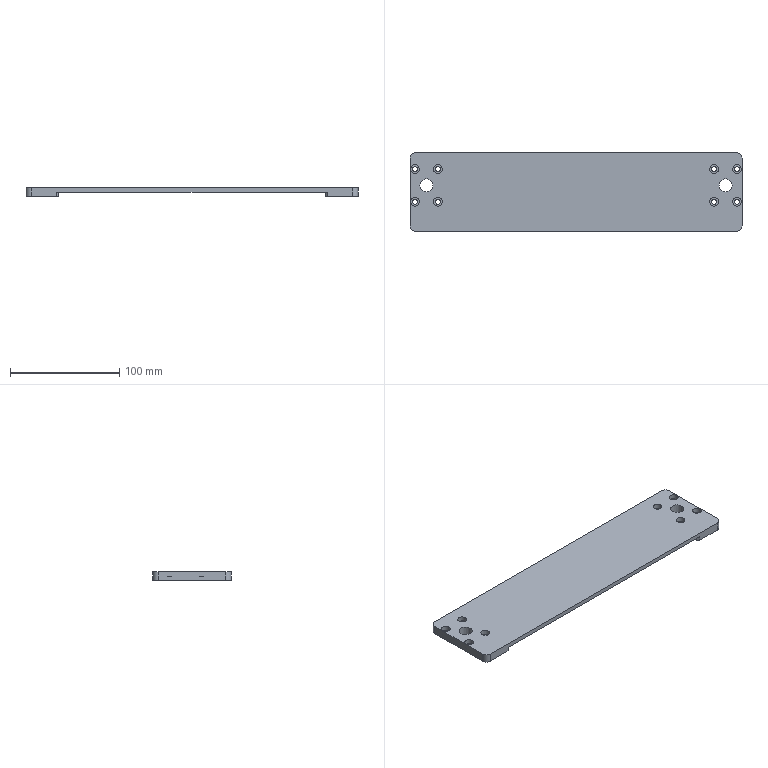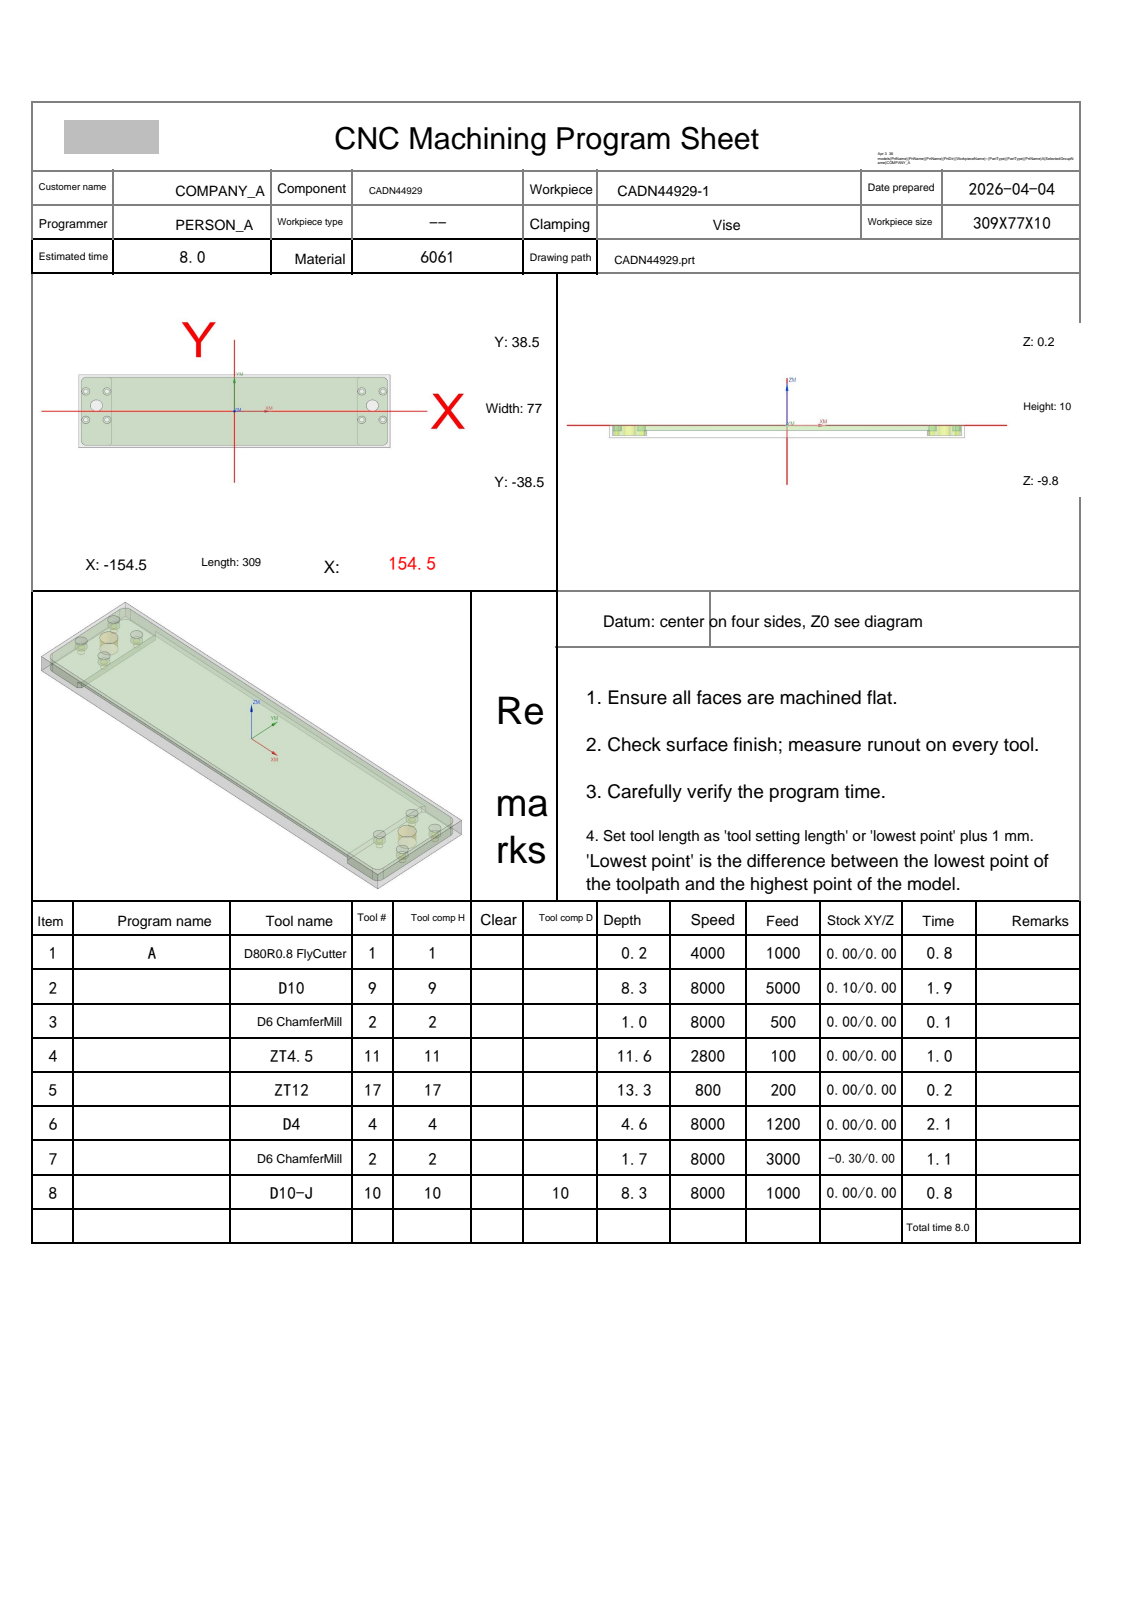NC program | NX | posted by the shop | part box 304 x 72 x 8 mm
Whole program:
%
O0001
(Machine time: 9.54 MIN)
(===Total Tool:7===)
(T1=D80R0.8 FlyCutter D=80.  R=0.8  D-  H01 Z=0.    )
(T9=D10     D=10.  R=0.   D-  H09 Z=-8.1  )
(T2=D6 ChamferMill   D=6.   R=0.   D-  H02 Z=-1.5  )
(T11=ZT4.5  D=4.5  DR_a=118 D-  H11 Z=-11.35)
(T17=ZT12   D=12.  DR_a=118 D-  H17 Z=-13.11)
(T4=D4      D=4.   R=0.   D4  H04 Z=-4.4  )
(T10=D10-J  D=10.  R=0.   D10 H10 Z=-8.1  )
G80 G90 G17 G49 G40
G91 G28 Z0
M01
N1 T01 M06
(D80R0.8 FlyCutter  D=80. R=0.8 H=01 ce=0.00 di=0.00)
G00 G90 G54 X-197. Y25.333 M03 S4000
G43 H01 Z20.
M08
Z2.
G01 Z0.0 F1000.
X-192.
X192.
Y-25.333
X-192.
X-197.
Z2.
G00 Z20.
G91 G28 Z0.0
M05
M09
G91 G28 Z0.0
M01
N2 T09 M06
(D10  D=10. R=0. H=09 ce=0.10 di=0.00)
G00 G90 G54 X0.0 Y-41.1 M03 S8000
G43 H09 Z20.
M08
Z.5
G01 X-147. Z.352 F5000.
G02 X-157.1 Y-31. Z.336 I0.0 J10.1
G01 Y31. Z.273
G02 X-147. Y41.1 Z.257 I10.1 J0.0
G01 X147. Z-.039
G02 X157.1 Y31. Z-.055 I0.0 J-10.1
G01 Y-31. Z-.118
G02 X147. Y-41.1 Z-.134 I-10.1 J0.0
G01 X-147. Z-.43
G02 X-157.1 Y-31. Z-.446 I0.0 J10.1
G01 Y31. Z-.509
G02 X-147. Y41.1 Z-.525 I10.1 J0.0
G01 X147. Z-.821
G02 X157.1 Y31. Z-.837 I0.0 J-10.1
G01 Y-31. Z-.899
G02 X147. Y-41.1 Z-.915 I-10.1 J0.0
G01 X-147. Z-1.212
G02 X-157.1 Y-31. Z-1.228 I0.0 J10.1
G01 Y31. Z-1.29
G02 X-147. Y41.1 Z-1.306 I10.1 J0.0
G01 X147. Z-1.603
G02 X157.1 Y31. Z-1.619 I0.0 J-10.1
G01 Y-31. Z-1.681
G02 X147. Y-41.1 Z-1.697 I-10.1 J0.0
G01 X-147. Z-1.994
G02 X-157.1 Y-31. Z-2.01 I0.0 J10.1
G01 Y31. Z-2.072
G02 X-147. Y41.1 Z-2.088 I10.1 J0.0
G01 X147. Z-2.385
G02 X157.1 Y31. Z-2.401 I0.0 J-10.1
G01 Y-31. Z-2.463
G02 X147. Y-41.1 Z-2.479 I-10.1 J0.0
G01 X-147. Z-2.775
G02 X-157.1 Y-31. Z-2.791 I0.0 J10.1
G01 Y31. Z-2.854
G02 X-147. Y41.1 Z-2.87 I10.1 J0.0
G01 X147. Z-3.166
G02 X157.1 Y31. Z-3.182 I0.0 J-10.1
G01 Y-31. Z-3.245
G02 X147. Y-41.1 Z-3.261 I-10.1 J0.0
G01 X-147. Z-3.557
G02 X-157.1 Y-31. Z-3.573 I0.0 J10.1
G01 Y31. Z-3.636
G02 X-147. Y41.1 Z-3.652 I10.1 J0.0
G01 X147. Z-3.948
G02 X157.1 Y31. Z-3.964 I0.0 J-10.1
G01 Y-31. Z-4.027
G02 X147. Y-41.1 Z-4.043 I-10.1 J0.0
G01 X-147. Z-4.339
G02 X-157.1 Y-31. Z-4.355 I0.0 J10.1
G01 Y31. Z-4.418
G02 X-147. Y41.1 Z-4.434 I10.1 J0.0
G01 X147. Z-4.73
G02 X157.1 Y31. Z-4.746 I0.0 J-10.1
G01 Y-31. Z-4.809
G02 X147. Y-41.1 Z-4.825 I-10.1 J0.0
G01 X-147. Z-5.121
G02 X-157.1 Y-31. Z-5.137 I0.0 J10.1
G01 Y31. Z-5.199
G02 X-147. Y41.1 Z-5.215 I10.1 J0.0
G01 X147. Z-5.512
G02 X157.1 Y31. Z-5.528 I0.0 J-10.1
G01 Y-31. Z-5.59
G02 X147. Y-41.1 Z-5.606 I-10.1 J0.0
G01 X-147. Z-5.903
G02 X-157.1 Y-31. Z-5.919 I0.0 J10.1
G01 Y31. Z-5.981
G02 X-147. Y41.1 Z-5.997 I10.1 J0.0
G01 X147. Z-6.294
G02 X157.1 Y31. Z-6.31 I0.0 J-10.1
G01 Y-31. Z-6.372
G02 X147. Y-41.1 Z-6.388 I-10.1 J0.0
G01 X-147. Z-6.685
G02 X-157.1 Y-31. Z-6.701 I0.0 J10.1
G01 Y31. Z-6.763
G02 X-147. Y41.1 Z-6.779 I10.1 J0.0
G01 X147. Z-7.075
G02 X157.1 Y31. Z-7.091 I0.0 J-10.1
G01 Y-31. Z-7.154
G02 X147. Y-41.1 Z-7.17 I-10.1 J0.0
G01 X-147. Z-7.466
G02 X-157.1 Y-31. Z-7.482 I0.0 J10.1
G01 Y31. Z-7.545
G02 X-147. Y41.1 Z-7.561 I10.1 J0.0
G01 X147. Z-7.857
G02 X157.1 Y31. Z-7.873 I0.0 J-10.1
G01 Y-31. Z-7.936
G02 X147. Y-41.1 Z-7.952 I-10.1 J0.0
G01 X0.0 Z-8.1
X-147.
G02 X-157.1 Y-31. I0.0 J10.1
G01 Y31.
G02 X-147. Y41.1 I10.1 J0.0
G01 X147.
G02 X157.1 Y31. I0.0 J-10.1
G01 Y-31.
G02 X147. Y-41.1 I-10.1 J0.0
G01 X0.0
X-.5
Z-7.1
G00 Z20.
G91 G28 Z0.0
M05
M09
G91 G28 Z0.0
M01
N3 T02 M06
(D6 ChamferMill  D=6. R=0. H=02 ce=0.00 di=0.00)
G00 G90 G54 X-126.5 Y-9. M03 S8000
G43 H02 Z20.
M08
G98 G81 X-126.5 Y-9. Z-.8 R1. F500.
X-147.5
X-137. Y6.
X-147.5 Y21.
X-126.5
X126.5
X147.5
X137. Y6.
X126.5 Y-9.
X147.5
G80
G00 Z20.
G91 G28 Z0.0
M05
M09
G91 G28 Z0.0
M01
N4 T11 M06
(ZT4.5 D=4.5 DR_a=118 H=11)
G00 G90 G54 X-126.5 Y21. M03 S2800
G43 H11 Z20.
M08
G98 G83 X-126.5 Y21. Z-11.352 R1. F100. Q2.
X-147.5
Y-9.
X-126.5
X126.5
X147.5
Y21.
X126.5
G80
G00 Z20.
G91 G28 Z0.0
M05
M09
G91 G28 Z0.0
M01
N5 T17 M06
(ZT12 D=12. DR_a=118 H=17)
G00 G90 G54 X-137. Y6. M03 S800
G43 H17 Z20.
M08
G98 G83 X-137. Y6. Z-13.105 R1. F200. Q2.
X137.
G80
G00 Z20.
G91 G28 Z0.0
M05
M09
G91 G28 Z0.0
M01
N6 T04 M06
(D4  D=4. R=0. H=04 ce=0.10 di=0.00)
G00 G90 G54 X-147.5 Y-9. M03 S8000
G43 H04 Z20.
M08
Z.5
G03 X-146.55 Y-9.95 I.95 J0.0 F1200.
X-145.6 Y-9. I0.0 J.95
X-145.6 Y-9. Z.2 I-1.9 J0.0
X-145.6 Y-9. Z-.1 I-1.9 J0.0
X-145.6 Y-9. Z-.4 I-1.9 J0.0
X-145.6 Y-9. Z-.7 I-1.9 J0.0
X-145.6 Y-9. Z-1. I-1.9 J0.0
X-145.6 Y-9. Z-1.3 I-1.9 J0.0
X-145.6 Y-9. Z-1.6 I-1.9 J0.0
X-145.6 Y-9. Z-1.9 I-1.9 J0.0
X-145.6 Y-9. Z-2.2 I-1.9 J0.0
X-145.6 Y-9. Z-2.5 I-1.9 J0.0
X-145.6 Y-9. Z-2.8 I-1.9 J0.0
X-145.6 Y-9. Z-3.1 I-1.9 J0.0
X-145.6 Y-9. Z-3.4 I-1.9 J0.0
X-145.6 Y-9. Z-3.7 I-1.9 J0.0
X-145.6 Y-9. Z-4. I-1.9 J0.0
X-145.6 Y-9. Z-4.3 I-1.9 J0.0
X-148.45 Y-7.355 Z-4.4 I-1.9 J0.0
X-149.4 Y-9. I.95 J-1.645
X-147.5 Y-10.9 I1.9 J0.0
X-145.6 Y-9. I0.0 J1.9
X-147.5 Y-7.1 I-1.9 J0.0
X-148.45 Y-7.355 I0.0 J-1.9
X-148.925 Y-8.177 I.475 J-.823
X-147.975 Y-9.127 I.95 J0.0
X-147.5 Y-9. I0.0 J.95
G00 Z20.
X-126.5
Z.5
G03 X-125.55 Y-9.95 I.95 J0.0
X-124.6 Y-9. I0.0 J.95
X-124.6 Y-9. Z.2 I-1.9 J0.0
X-124.6 Y-9. Z-.1 I-1.9 J0.0
X-124.6 Y-9. Z-.4 I-1.9 J0.0
X-124.6 Y-9. Z-.7 I-1.9 J0.0
X-124.6 Y-9. Z-1. I-1.9 J0.0
X-124.6 Y-9. Z-1.3 I-1.9 J0.0
X-124.6 Y-9. Z-1.6 I-1.9 J0.0
X-124.6 Y-9. Z-1.9 I-1.9 J0.0
X-124.6 Y-9. Z-2.2 I-1.9 J0.0
X-124.6 Y-9. Z-2.5 I-1.9 J0.0
X-124.6 Y-9. Z-2.8 I-1.9 J0.0
X-124.6 Y-9. Z-3.1 I-1.9 J0.0
X-124.6 Y-9. Z-3.4 I-1.9 J0.0
X-124.6 Y-9. Z-3.7 I-1.9 J0.0
X-124.6 Y-9. Z-4. I-1.9 J0.0
X-124.6 Y-9. Z-4.3 I-1.9 J0.0
X-127.45 Y-7.355 Z-4.4 I-1.9 J0.0
X-128.4 Y-9. I.95 J-1.645
X-126.5 Y-10.9 I1.9 J0.0
X-124.6 Y-9. I0.0 J1.9
X-126.5 Y-7.1 I-1.9 J0.0
X-127.45 Y-7.355 I0.0 J-1.9
X-127.925 Y-8.177 I.475 J-.823
X-126.975 Y-9.127 I.95 J0.0
X-126.5 Y-9. I0.0 J.95
G00 Z20.
X-147.5 Y21.
Z.5
G03 X-146.55 Y20.05 I.95 J0.0
X-145.6 Y21. I0.0 J.95
X-145.6 Y21. Z.2 I-1.9 J0.0
X-145.6 Y21. Z-.1 I-1.9 J0.0
X-145.6 Y21. Z-.4 I-1.9 J0.0
X-145.6 Y21. Z-.7 I-1.9 J0.0
X-145.6 Y21. Z-1. I-1.9 J0.0
X-145.6 Y21. Z-1.3 I-1.9 J0.0
X-145.6 Y21. Z-1.6 I-1.9 J0.0
X-145.6 Y21. Z-1.9 I-1.9 J0.0
X-145.6 Y21. Z-2.2 I-1.9 J0.0
X-145.6 Y21. Z-2.5 I-1.9 J0.0
X-145.6 Y21. Z-2.8 I-1.9 J0.0
X-145.6 Y21. Z-3.1 I-1.9 J0.0
X-145.6 Y21. Z-3.4 I-1.9 J0.0
X-145.6 Y21. Z-3.7 I-1.9 J0.0
X-145.6 Y21. Z-4. I-1.9 J0.0
X-145.6 Y21. Z-4.3 I-1.9 J0.0
X-148.45 Y22.645 Z-4.4 I-1.9 J0.0
X-149.4 Y21. I.95 J-1.645
X-147.5 Y19.1 I1.9 J0.0
X-145.6 Y21. I0.0 J1.9
X-147.5 Y22.9 I-1.9 J0.0
X-148.45 Y22.645 I0.0 J-1.9
X-148.925 Y21.823 I.475 J-.823
X-147.975 Y20.873 I.95 J0.0
X-147.5 Y21. I0.0 J.95
G00 Z20.
X-126.5
Z.5
G03 X-125.55 Y20.05 I.95 J0.0
X-124.6 Y21. I0.0 J.95
X-124.6 Y21. Z.2 I-1.9 J0.0
X-124.6 Y21. Z-.1 I-1.9 J0.0
X-124.6 Y21. Z-.4 I-1.9 J0.0
X-124.6 Y21. Z-.7 I-1.9 J0.0
X-124.6 Y21. Z-1. I-1.9 J0.0
X-124.6 Y21. Z-1.3 I-1.9 J0.0
X-124.6 Y21. Z-1.6 I-1.9 J0.0
X-124.6 Y21. Z-1.9 I-1.9 J0.0
X-124.6 Y21. Z-2.2 I-1.9 J0.0
X-124.6 Y21. Z-2.5 I-1.9 J0.0
X-124.6 Y21. Z-2.8 I-1.9 J0.0
X-124.6 Y21. Z-3.1 I-1.9 J0.0
X-124.6 Y21. Z-3.4 I-1.9 J0.0
X-124.6 Y21. Z-3.7 I-1.9 J0.0
X-124.6 Y21. Z-4. I-1.9 J0.0
X-124.6 Y21. Z-4.3 I-1.9 J0.0
X-127.45 Y22.645 Z-4.4 I-1.9 J0.0
X-128.4 Y21. I.95 J-1.645
X-126.5 Y19.1 I1.9 J0.0
X-124.6 Y21. I0.0 J1.9
X-126.5 Y22.9 I-1.9 J0.0
X-127.45 Y22.645 I0.0 J-1.9
X-127.925 Y21.823 I.475 J-.823
X-126.975 Y20.873 I.95 J0.0
X-126.5 Y21. I0.0 J.95
G00 Z20.
X126.5
Z.5
G03 X127.45 Y20.05 I.95 J0.0
X128.4 Y21. I0.0 J.95
X128.4 Y21. Z.2 I-1.9 J0.0
X128.4 Y21. Z-.1 I-1.9 J0.0
X128.4 Y21. Z-.4 I-1.9 J0.0
X128.4 Y21. Z-.7 I-1.9 J0.0
X128.4 Y21. Z-1. I-1.9 J0.0
X128.4 Y21. Z-1.3 I-1.9 J0.0
X128.4 Y21. Z-1.6 I-1.9 J0.0
X128.4 Y21. Z-1.9 I-1.9 J0.0
X128.4 Y21. Z-2.2 I-1.9 J0.0
X128.4 Y21. Z-2.5 I-1.9 J0.0
X128.4 Y21. Z-2.8 I-1.9 J0.0
X128.4 Y21. Z-3.1 I-1.9 J0.0
X128.4 Y21. Z-3.4 I-1.9 J0.0
X128.4 Y21. Z-3.7 I-1.9 J0.0
X128.4 Y21. Z-4. I-1.9 J0.0
X128.4 Y21. Z-4.3 I-1.9 J0.0
X125.55 Y22.645 Z-4.4 I-1.9 J0.0
X124.6 Y21. I.95 J-1.645
X126.5 Y19.1 I1.9 J0.0
X128.4 Y21. I0.0 J1.9
X126.5 Y22.9 I-1.9 J0.0
X125.55 Y22.645 I0.0 J-1.9
X125.075 Y21.823 I.475 J-.823
X126.025 Y20.873 I.95 J0.0
X126.5 Y21. I0.0 J.95
G00 Z20.
X147.5
Z.5
G03 X148.45 Y20.05 I.95 J0.0
X149.4 Y21. I0.0 J.95
X149.4 Y21. Z.2 I-1.9 J0.0
X149.4 Y21. Z-.1 I-1.9 J0.0
X149.4 Y21. Z-.4 I-1.9 J0.0
X149.4 Y21. Z-.7 I-1.9 J0.0
X149.4 Y21. Z-1. I-1.9 J0.0
X149.4 Y21. Z-1.3 I-1.9 J0.0
X149.4 Y21. Z-1.6 I-1.9 J0.0
X149.4 Y21. Z-1.9 I-1.9 J0.0
X149.4 Y21. Z-2.2 I-1.9 J0.0
X149.4 Y21. Z-2.5 I-1.9 J0.0
X149.4 Y21. Z-2.8 I-1.9 J0.0
X149.4 Y21. Z-3.1 I-1.9 J0.0
X149.4 Y21. Z-3.4 I-1.9 J0.0
X149.4 Y21. Z-3.7 I-1.9 J0.0
X149.4 Y21. Z-4. I-1.9 J0.0
X149.4 Y21. Z-4.3 I-1.9 J0.0
X146.55 Y22.645 Z-4.4 I-1.9 J0.0
X145.6 Y21. I.95 J-1.645
X147.5 Y19.1 I1.9 J0.0
X149.4 Y21. I0.0 J1.9
X147.5 Y22.9 I-1.9 J0.0
X146.55 Y22.645 I0.0 J-1.9
X146.075 Y21.823 I.475 J-.823
X147.025 Y20.873 I.95 J0.0
X147.5 Y21. I0.0 J.95
G00 Z20.
Y-9.
Z.5
G03 X148.45 Y-9.95 I.95 J0.0
X149.4 Y-9. I0.0 J.95
X149.4 Y-9. Z.2 I-1.9 J0.0
X149.4 Y-9. Z-.1 I-1.9 J0.0
X149.4 Y-9. Z-.4 I-1.9 J0.0
X149.4 Y-9. Z-.7 I-1.9 J0.0
X149.4 Y-9. Z-1. I-1.9 J0.0
X149.4 Y-9. Z-1.3 I-1.9 J0.0
X149.4 Y-9. Z-1.6 I-1.9 J0.0
X149.4 Y-9. Z-1.9 I-1.9 J0.0
X149.4 Y-9. Z-2.2 I-1.9 J0.0
X149.4 Y-9. Z-2.5 I-1.9 J0.0
X149.4 Y-9. Z-2.8 I-1.9 J0.0
X149.4 Y-9. Z-3.1 I-1.9 J0.0
X149.4 Y-9. Z-3.4 I-1.9 J0.0
X149.4 Y-9. Z-3.7 I-1.9 J0.0
X149.4 Y-9. Z-4. I-1.9 J0.0
X149.4 Y-9. Z-4.3 I-1.9 J0.0
X146.55 Y-7.355 Z-4.4 I-1.9 J0.0
X145.6 Y-9. I.95 J-1.645
X147.5 Y-10.9 I1.9 J0.0
X149.4 Y-9. I0.0 J1.9
X147.5 Y-7.1 I-1.9 J0.0
X146.55 Y-7.355 I0.0 J-1.9
X146.075 Y-8.177 I.475 J-.823
X147.025 Y-9.127 I.95 J0.0
X147.5 Y-9. I0.0 J.95
G00 Z20.
X126.5
Z.5
G03 X127.45 Y-9.95 I.95 J0.0
X128.4 Y-9. I0.0 J.95
X128.4 Y-9. Z.2 I-1.9 J0.0
X128.4 Y-9. Z-.1 I-1.9 J0.0
X128.4 Y-9. Z-.4 I-1.9 J0.0
X128.4 Y-9. Z-.7 I-1.9 J0.0
X128.4 Y-9. Z-1. I-1.9 J0.0
X128.4 Y-9. Z-1.3 I-1.9 J0.0
X128.4 Y-9. Z-1.6 I-1.9 J0.0
X128.4 Y-9. Z-1.9 I-1.9 J0.0
X128.4 Y-9. Z-2.2 I-1.9 J0.0
X128.4 Y-9. Z-2.5 I-1.9 J0.0
X128.4 Y-9. Z-2.8 I-1.9 J0.0
X128.4 Y-9. Z-3.1 I-1.9 J0.0
X128.4 Y-9. Z-3.4 I-1.9 J0.0
X128.4 Y-9. Z-3.7 I-1.9 J0.0
X128.4 Y-9. Z-4. I-1.9 J0.0
X128.4 Y-9. Z-4.3 I-1.9 J0.0
X125.55 Y-7.355 Z-4.4 I-1.9 J0.0
X124.6 Y-9. I.95 J-1.645
X126.5 Y-10.9 I1.9 J0.0
X128.4 Y-9. I0.0 J1.9
X126.5 Y-7.1 I-1.9 J0.0
X125.55 Y-7.355 I0.0 J-1.9
X125.075 Y-8.177 I.475 J-.823
X126.025 Y-9.127 I.95 J0.0
X126.5 Y-9. I0.0 J.95
G00 Z20.
G00 G90 X-147.5 Y-9. M03 S8000
Z20.
Z.5
G41 D04
G01 X-147.46 Y-9.196 F500.
G03 X-146.49 Y-9.99 I.97 J.196
X-145.5 Y-9. I0.0 J.99
X-145.516 Y-9.251 Z-4.4 I-2. J0.0
X-145.5 Y-9. I-1.984 J.251
X-147.5 Y-7. I-2. J0.0
X-149.5 Y-9. I0.0 J-2.
X-147.5 Y-11. I2. J0.0
X-145.516 Y-9.251 I0.0 J2.
G01 X-145.508 Y-9.127
G03 X-146.498 Y-8.137 I-.99 J0.0
X-147.436 Y-8.81 I0.0 J-.99
G01 G40 X-147.5 Y-9.
G00 Z20.
X-126.5
Z.5
G41 D04
G01 X-126.46 Y-9.196
G03 X-125.49 Y-9.99 I.97 J.196
X-124.5 Y-9. I0.0 J.99
X-124.516 Y-9.251 Z-4.4 I-2. J0.0
X-124.5 Y-9. I-1.984 J.251
X-126.5 Y-7. I-2. J0.0
X-128.5 Y-9. I0.0 J-2.
X-126.5 Y-11. I2. J0.0
X-124.516 Y-9.251 I0.0 J2.
G01 X-124.508 Y-9.127
G03 X-125.498 Y-8.137 I-.99 J0.0
X-126.436 Y-8.81 I0.0 J-.99
G01 G40 X-126.5 Y-9.
G00 Z20.
X-147.5 Y21.
Z.5
G41 D04
G01 X-147.46 Y20.804
G03 X-146.49 Y20.01 I.97 J.196
X-145.5 Y21. I0.0 J.99
X-145.516 Y20.749 Z-4.4 I-2. J0.0
X-145.5 Y21. I-1.984 J.251
X-147.5 Y23. I-2. J0.0
X-149.5 Y21. I0.0 J-2.
X-147.5 Y19. I2. J0.0
X-145.516 Y20.749 I0.0 J2.
G01 X-145.508 Y20.873
G03 X-146.498 Y21.863 I-.99 J0.0
X-147.436 Y21.19 I0.0 J-.99
G01 G40 X-147.5 Y21.
G00 Z20.
X-126.5
Z.5
G41 D04
G01 X-126.46 Y20.804
G03 X-125.49 Y20.01 I.97 J.196
X-124.5 Y21. I0.0 J.99
X-124.516 Y20.749 Z-4.4 I-2. J0.0
X-124.5 Y21. I-1.984 J.251
X-126.5 Y23. I-2. J0.0
X-128.5 Y21. I0.0 J-2.
X-126.5 Y19. I2. J0.0
X-124.516 Y20.749 I0.0 J2.
G01 X-124.508 Y20.873
G03 X-125.498 Y21.863 I-.99 J0.0
X-126.436 Y21.19 I0.0 J-.99
G01 G40 X-126.5 Y21.
G00 Z20.
X126.5
Z.5
G41 D04
G01 X126.54 Y20.804
G03 X127.51 Y20.01 I.97 J.196
X128.5 Y21. I0.0 J.99
X128.484 Y20.749 Z-4.4 I-2. J0.0
X128.5 Y21. I-1.984 J.251
X126.5 Y23. I-2. J0.0
X124.5 Y21. I0.0 J-2.
X126.5 Y19. I2. J0.0
X128.484 Y20.749 I0.0 J2.
G01 X128.492 Y20.873
G03 X127.502 Y21.863 I-.99 J0.0
X126.564 Y21.19 I0.0 J-.99
G01 G40 X126.5 Y21.
G00 Z20.
X147.5
Z.5
G41 D04
G01 X147.54 Y20.804
G03 X148.51 Y20.01 I.97 J.196
X149.5 Y21. I0.0 J.99
X149.484 Y20.749 Z-4.4 I-2. J0.0
X149.5 Y21. I-1.984 J.251
X147.5 Y23. I-2. J0.0
X145.5 Y21. I0.0 J-2.
X147.5 Y19. I2. J0.0
X149.484 Y20.749 I0.0 J2.
G01 X149.492 Y20.873
G03 X148.502 Y21.863 I-.99 J0.0
X147.564 Y21.19 I0.0 J-.99
G01 G40 X147.5 Y21.
G00 Z20.
Y-9.
Z.5
G41 D04
G01 X147.54 Y-9.196
G03 X148.51 Y-9.99 I.97 J.196
X149.5 Y-9. I0.0 J.99
X149.484 Y-9.251 Z-4.4 I-2. J0.0
X149.5 Y-9. I-1.984 J.251
X147.5 Y-7. I-2. J0.0
X145.5 Y-9. I0.0 J-2.
X147.5 Y-11. I2. J0.0
X149.484 Y-9.251 I0.0 J2.
G01 X149.492 Y-9.127
G03 X148.502 Y-8.137 I-.99 J0.0
X147.564 Y-8.81 I0.0 J-.99
G01 G40 X147.5 Y-9.
G00 Z20.
X126.5
Z.5
G41 D04
G01 X126.54 Y-9.196
G03 X127.51 Y-9.99 I.97 J.196
X128.5 Y-9. I0.0 J.99
X128.484 Y-9.251 Z-4.4 I-2. J0.0
X128.5 Y-9. I-1.984 J.251
X126.5 Y-7. I-2. J0.0
X124.5 Y-9. I0.0 J-2.
X126.5 Y-11. I2. J0.0
X128.484 Y-9.251 I0.0 J2.
G01 X128.492 Y-9.127
G03 X127.502 Y-8.137 I-.99 J0.0
X126.564 Y-8.81 I0.0 J-.99
G01 G40 X126.5 Y-9.
G00 Z20.
G91 G28 Z0.0
M05
M09
G91 G28 Z0.0
M01
N7 T02 M06
(D6 ChamferMill  D=6. R=0. H=02 ce=0.00 di=0.00)
G00 G90 G54 X.25 Y-38.128 M03 S8000
G43 H02 Z20.
M08
Z2.099
G01 Z-1.5 F3000.
G03 X.33 Y-37.828 I-.52 J.3
X.03 Y-37.308 I-.6 J0.0
G01 X0.0 Y-37.3
X-147.
G02 X-153.3 Y-31. I0.0 J6.3
G01 Y31.
G02 X-147. Y37.3 I6.3 J0.0
G01 X147.
G02 X153.3 Y31. I0.0 J-6.3
G01 Y-31.
G02 X147. Y-37.3 I-6.3 J0.0
G01 X0.0
X-.03 Y-37.308
G03 X-.33 Y-37.828 I.3 J-.52
X-.25 Y-38.128 I.6 J0.0
G01 Z2.099
G00 Z20.
G00 G90 X-129.712 Y20.253 M03 S8000
Z20.
Z2.5
G01 X-129.66 Y20.038 Z2.42 F500.
X-129.524 Y19.672 Z2.278
X-129.347 Y19.325 Z2.136
X-129.129 Y19.001 Z1.994
X-128.875 Y18.705 Z1.852
X-128.588 Y18.441 Z1.71
X-128.272 Y18.212 Z1.568
X-128.028 Y18.072 Z1.465
X-127.672 Y17.912 Z1.323
X-127.3 Y17.795 Z1.181
X-126.916 Y17.723 Z1.039
X-126.527 Y17.697 Z.897
X-126.138 Y17.717 Z.755
X-125.753 Y17.783 Z.613
X-125.379 Y17.893 Z.471
X-125.02 Y18.047 Z.329
X-124.682 Y18.242 Z.187
X-124.37 Y18.476 Z.045
X-124.087 Y18.744 Z-.097
X-123.838 Y19.045 Z-.239
X-123.626 Y19.372 Z-.381
X-123.454 Y19.722 Z-.523
X-123.325 Y20.09 Z-.665
X-123.24 Y20.471 Z-.807
X-123.2 Y20.859 Z-.949
Y21. Z-1.
G03 X-126.5 Y24.3 I-3.3 J0.0
X-129.8 Y21. I0.0 J-3.3
X-126.5 Y17.7 I3.3 J0.0
X-123.2 Y21. I0.0 J3.3
X-123.238 Y21.498 I-3.3 J0.0
G01 Z1.5
G00 Z20.
X-150.712 Y20.253
Z2.5
G01 X-150.66 Y20.038 Z2.42
X-150.524 Y19.672 Z2.278
X-150.347 Y19.325 Z2.136
X-150.129 Y19.001 Z1.994
X-149.875 Y18.705 Z1.852
X-149.588 Y18.441 Z1.71
X-149.272 Y18.212 Z1.568
X-149.028 Y18.072 Z1.465
X-148.672 Y17.912 Z1.323
X-148.3 Y17.795 Z1.181
X-147.916 Y17.723 Z1.039
X-147.527 Y17.697 Z.897
X-147.138 Y17.717 Z.755
X-146.753 Y17.783 Z.613
X-146.379 Y17.893 Z.471
X-146.02 Y18.047 Z.329
X-145.682 Y18.242 Z.187
X-145.37 Y18.476 Z.045
X-145.087 Y18.744 Z-.097
X-144.838 Y19.045 Z-.239
X-144.626 Y19.372 Z-.381
X-144.454 Y19.722 Z-.523
X-144.325 Y20.09 Z-.665
X-144.24 Y20.471 Z-.807
X-144.2 Y20.859 Z-.949
Y21. Z-1.
G03 X-147.5 Y24.3 I-3.3 J0.0
X-150.8 Y21. I0.0 J-3.3
X-147.5 Y17.7 I3.3 J0.0
X-144.2 Y21. I0.0 J3.3
X-144.238 Y21.498 I-3.3 J0.0
G01 Z1.5
G00 Z20.
X-150.712 Y-9.747
Z2.5
G01 X-150.66 Y-9.962 Z2.42
X-150.524 Y-10.328 Z2.278
X-150.347 Y-10.675 Z2.136
X-150.129 Y-10.999 Z1.994
X-149.875 Y-11.295 Z1.852
X-149.588 Y-11.559 Z1.71
X-149.272 Y-11.788 Z1.568
X-149.028 Y-11.928 Z1.465
X-148.672 Y-12.088 Z1.323
X-148.3 Y-12.205 Z1.181
X-147.916 Y-12.277 Z1.039
X-147.527 Y-12.303 Z.897
X-147.138 Y-12.283 Z.755
X-146.753 Y-12.217 Z.613
X-146.379 Y-12.107 Z.471
X-146.02 Y-11.953 Z.329
X-145.682 Y-11.758 Z.187
X-145.37 Y-11.524 Z.045
X-145.087 Y-11.256 Z-.097
X-144.838 Y-10.955 Z-.239
X-144.626 Y-10.628 Z-.381
X-144.454 Y-10.278 Z-.523
X-144.325 Y-9.91 Z-.665
X-144.24 Y-9.529 Z-.807
X-144.2 Y-9.141 Z-.949
Y-9. Z-1.
G03 X-147.5 Y-5.7 I-3.3 J0.0
X-150.8 Y-9. I0.0 J-3.3
X-147.5 Y-12.3 I3.3 J0.0
X-144.2 Y-9. I0.0 J3.3
X-144.238 Y-8.502 I-3.3 J0.0
G01 Z1.5
G00 Z20.
X-129.712 Y-9.747
Z2.5
G01 X-129.66 Y-9.962 Z2.42
X-129.524 Y-10.328 Z2.278
X-129.347 Y-10.675 Z2.136
X-129.129 Y-10.999 Z1.994
X-128.875 Y-11.295 Z1.852
X-128.588 Y-11.559 Z1.71
X-128.272 Y-11.788 Z1.568
X-128.028 Y-11.928 Z1.465
X-127.672 Y-12.088 Z1.323
X-127.3 Y-12.205 Z1.181
X-126.916 Y-12.277 Z1.039
X-126.527 Y-12.303 Z.897
X-126.138 Y-12.283 Z.755
X-125.753 Y-12.217 Z.613
X-125.379 Y-12.107 Z.471
X-125.02 Y-11.953 Z.329
X-124.682 Y-11.758 Z.187
X-124.37 Y-11.524 Z.045
X-124.087 Y-11.256 Z-.097
X-123.838 Y-10.955 Z-.239
X-123.626 Y-10.628 Z-.381
X-123.454 Y-10.278 Z-.523
X-123.325 Y-9.91 Z-.665
X-123.24 Y-9.529 Z-.807
X-123.2 Y-9.141 Z-.949
Y-9. Z-1.
G03 X-126.5 Y-5.7 I-3.3 J0.0
X-129.8 Y-9. I0.0 J-3.3
X-126.5 Y-12.3 I3.3 J0.0
X-123.2 Y-9. I0.0 J3.3
X-123.238 Y-8.502 I-3.3 J0.0
G01 Z1.5
G00 Z20.
X123.288 Y-9.747
Z2.5
G01 X123.34 Y-9.962 Z2.42
X123.476 Y-10.328 Z2.278
X123.653 Y-10.675 Z2.136
X123.871 Y-10.999 Z1.994
X124.125 Y-11.295 Z1.852
X124.412 Y-11.559 Z1.71
X124.728 Y-11.788 Z1.568
X124.972 Y-11.928 Z1.465
X125.328 Y-12.088 Z1.323
X125.7 Y-12.205 Z1.181
X126.084 Y-12.277 Z1.039
X126.473 Y-12.303 Z.897
X126.862 Y-12.283 Z.755
X127.247 Y-12.217 Z.613
X127.621 Y-12.107 Z.471
X127.98 Y-11.953 Z.329
X128.318 Y-11.758 Z.187
X128.63 Y-11.524 Z.045
X128.913 Y-11.256 Z-.097
X129.162 Y-10.955 Z-.239
X129.374 Y-10.628 Z-.381
X129.546 Y-10.278 Z-.523
X129.675 Y-9.91 Z-.665
X129.76 Y-9.529 Z-.807
X129.8 Y-9.141 Z-.949
Y-9. Z-1.
G03 X126.5 Y-5.7 I-3.3 J0.0
X123.2 Y-9. I0.0 J-3.3
X126.5 Y-12.3 I3.3 J0.0
X129.8 Y-9. I0.0 J3.3
X129.762 Y-8.502 I-3.3 J0.0
G01 Z1.5
G00 Z20.
X144.288 Y-9.747
Z2.5
G01 X144.34 Y-9.962 Z2.42
X144.476 Y-10.328 Z2.278
X144.653 Y-10.675 Z2.136
X144.871 Y-10.999 Z1.994
X145.125 Y-11.295 Z1.852
X145.412 Y-11.559 Z1.71
X145.728 Y-11.788 Z1.568
X145.972 Y-11.928 Z1.465
X146.328 Y-12.088 Z1.323
X146.7 Y-12.205 Z1.181
X147.084 Y-12.277 Z1.039
X147.473 Y-12.303 Z.897
X147.862 Y-12.283 Z.755
X148.247 Y-12.217 Z.613
X148.621 Y-12.107 Z.471
X148.98 Y-11.953 Z.329
X149.318 Y-11.758 Z.187
X149.63 Y-11.524 Z.045
X149.913 Y-11.256 Z-.097
X150.162 Y-10.955 Z-.239
X150.374 Y-10.628 Z-.381
X150.546 Y-10.278 Z-.523
X150.675 Y-9.91 Z-.665
X150.76 Y-9.529 Z-.807
X150.8 Y-9.141 Z-.949
Y-9. Z-1.
G03 X147.5 Y-5.7 I-3.3 J0.0
X144.2 Y-9. I0.0 J-3.3
X147.5 Y-12.3 I3.3 J0.0
X150.8 Y-9. I0.0 J3.3
X150.762 Y-8.502 I-3.3 J0.0
G01 Z1.5
G00 Z20.
X144.288 Y20.253
Z2.5
G01 X144.34 Y20.038 Z2.42
X144.476 Y19.672 Z2.278
X144.653 Y19.325 Z2.136
X144.871 Y19.001 Z1.994
X145.125 Y18.705 Z1.852
X145.412 Y18.441 Z1.71
X145.728 Y18.212 Z1.568
X145.972 Y18.072 Z1.465
X146.328 Y17.912 Z1.323
X146.7 Y17.795 Z1.181
X147.084 Y17.723 Z1.039
X147.473 Y17.697 Z.897
X147.862 Y17.717 Z.755
X148.247 Y17.783 Z.613
X148.621 Y17.893 Z.471
X148.98 Y18.047 Z.329
X149.318 Y18.242 Z.187
X149.63 Y18.476 Z.045
X149.913 Y18.744 Z-.097
X150.162 Y19.045 Z-.239
X150.374 Y19.372 Z-.381
X150.546 Y19.722 Z-.523
X150.675 Y20.09 Z-.665
X150.76 Y20.471 Z-.807
X150.8 Y20.859 Z-.949
Y21. Z-1.
G03 X147.5 Y24.3 I-3.3 J0.0
X144.2 Y21. I0.0 J-3.3
X147.5 Y17.7 I3.3 J0.0
X150.8 Y21. I0.0 J3.3
X150.762 Y21.498 I-3.3 J0.0
G01 Z1.5
G00 Z20.
X123.288 Y20.253
Z2.5
G01 X123.34 Y20.038 Z2.42
X123.476 Y19.672 Z2.278
X123.653 Y19.325 Z2.136
X123.871 Y19.001 Z1.994
X124.125 Y18.705 Z1.852
X124.412 Y18.441 Z1.71
X124.728 Y18.212 Z1.568
X124.972 Y18.072 Z1.465
X125.328 Y17.912 Z1.323
X125.7 Y17.795 Z1.181
X126.084 Y17.723 Z1.039
X126.473 Y17.697 Z.897
X126.862 Y17.717 Z.755
X127.247 Y17.783 Z.613
X127.621 Y17.893 Z.471
X127.98 Y18.047 Z.329
X128.318 Y18.242 Z.187
X128.63 Y18.476 Z.045
X128.913 Y18.744 Z-.097
X129.162 Y19.045 Z-.239
X129.374 Y19.372 Z-.381
X129.546 Y19.722 Z-.523
X129.675 Y20.09 Z-.665
X129.76 Y20.471 Z-.807
X129.8 Y20.859 Z-.949
Y21. Z-1.
G03 X126.5 Y24.3 I-3.3 J0.0
X123.2 Y21. I0.0 J-3.3
X126.5 Y17.7 I3.3 J0.0
X129.8 Y21. I0.0 J3.3
X129.762 Y21.498 I-3.3 J0.0
G01 Z1.5
G00 Z20.
G00 G90 X-139.3 Y9. M03 S8000
Z20.
Z-.5
G01 Z-1. F500.
G03 X-142.3 Y6. I0.0 J-3.
X-137. Y.7 I5.3 J0.0
X-131.7 Y6. I0.0 J5.3
X-137. Y11.3 I-5.3 J0.0
X-142.3 Y6. I0.0 J-5.3
X-139.3 Y3. I3. J0.0
G01 Z-.5
G00 Z20.
X134.7 Y9.
Z-.5
G01 Z-1.
G03 X131.7 Y6. I0.0 J-3.
X137. Y.7 I5.3 J0.0
X142.3 Y6. I0.0 J5.3
X137. Y11.3 I-5.3 J0.0
X131.7 Y6. I0.0 J-5.3
X134.7 Y3. I3. J0.0
G01 Z-.5
G00 Z20.
G91 G28 Z0.0
M05
M09
G91 G28 Z0.0
M01
N8 T10 M06
(D10-J  D=10. R=0. H=10 ce=0.00 di=0.00)
G00 G90 G54 X148.008 Y-42.154 M03 S8000
G43 H10 Z20.
M08
Z-7.6
G01 Z-8.1 F1000.
G41 D10
X147.999 Y-41.955
G03 X147. Y-41. I-.999 J-.045
G01 X-147.
G02 X-157. Y-31. I0.0 J10.
G01 Y31.
G02 X-147. Y41. I10. J0.0
G01 X147.
G02 X157. Y31. I0.0 J-10.
G01 Y-31.
G02 X147. Y-41. I-10. J0.0
G01 X146.5
G03 X145.5 Y-42. I0.0 J-1.
G01 G40 Y-42.2
Z-7.6
G00 Z20.
M05
M09
G91 G28 Z0.0
G91 G28 Y0.0
M30
%